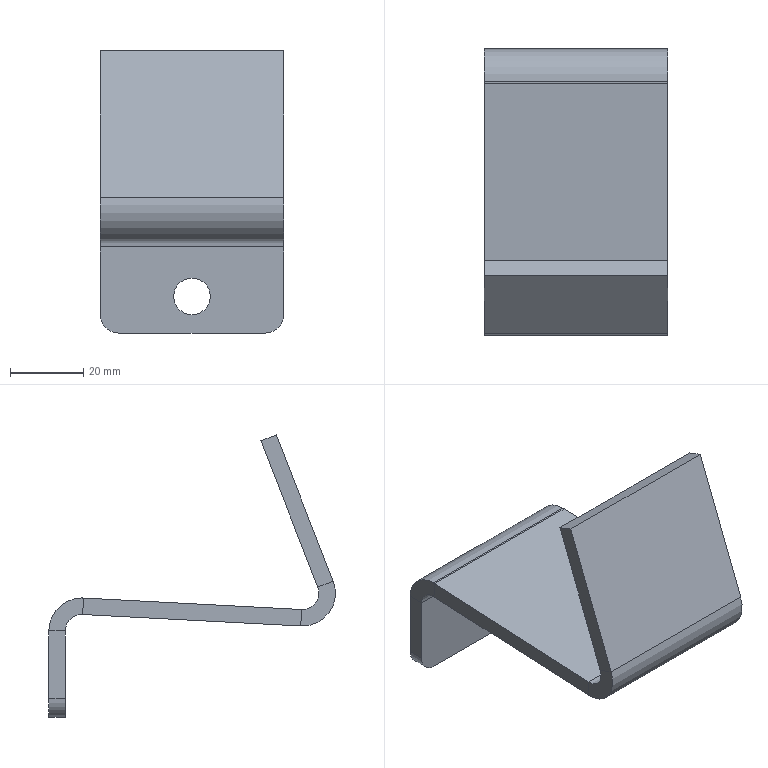Part | SolidWorks | features Fillet 1, FlatPattern 1, ICE 1, SMBaseFlange 1, SheetMetal 1 | 1 solid | 28 faces | box 50 x 78.274 x 77.035 mm | volume 33443 mm3 | plane 18 | cylinder 10 | commonest cylinder face diameters 10 x4 9 x3 18 x3
STEP:
#1=CARTESIAN_POINT('',(0.,-4.5,5.));
#2=VERTEX_POINT('',#1);
#3=CARTESIAN_POINT('',(0.,-4.5,15.));
#4=VERTEX_POINT('',#3);
#5=CARTESIAN_POINT('',(0.,-4.5,10.));
#6=DIRECTION('',(0.,1.,0.));
#7=DIRECTION('',(0.,0.,-1.));
#8=AXIS2_PLACEMENT_3D('',#5,#6,#7);
#9=CIRCLE('',#8,5.);
#10=EDGE_CURVE('',#2,#4,#9,.T.);
#11=ORIENTED_EDGE('',*,*,#10,.F.);
#12=CARTESIAN_POINT('',(0.,0.,5.));
#13=VERTEX_POINT('',#12);
#14=CARTESIAN_POINT('',(0.,-78.275,5.));
#15=DIRECTION('',(0.,1.,0.));
#16=VECTOR('',#15,1000.);
#17=LINE('',#14,#16);
#18=EDGE_CURVE('',#2,#13,#17,.T.);
#19=ORIENTED_EDGE('',*,*,#18,.T.);
#20=CARTESIAN_POINT('',(0.,0.,15.));
#21=VERTEX_POINT('',#20);
#22=CARTESIAN_POINT('',(0.,0.,10.));
#23=DIRECTION('',(0.,1.,0.));
#24=DIRECTION('',(0.,0.,1.));
#25=AXIS2_PLACEMENT_3D('',#22,#23,#24);
#26=CIRCLE('',#25,5.);
#27=EDGE_CURVE('',#13,#21,#26,.T.);
#28=ORIENTED_EDGE('',*,*,#27,.T.);
#29=CARTESIAN_POINT('',(0.,-78.275,15.));
#30=DIRECTION('',(0.,1.,0.));
#31=VECTOR('',#30,1000.);
#32=LINE('',#29,#31);
#33=EDGE_CURVE('',#4,#21,#32,.T.);
#34=ORIENTED_EDGE('',*,*,#33,.F.);
#35=EDGE_LOOP('',(#11,#19,#28,#34));
#36=FACE_OUTER_BOUND('',#35,.T.);
#37=CARTESIAN_POINT('',(0.,-78.275,10.));
#38=DIRECTION('',(0.,1.,0.));
#39=DIRECTION('',(0.,0.,1.));
#40=AXIS2_PLACEMENT_3D('',#37,#38,#39);
#41=CYLINDRICAL_SURFACE('',#40,5.);
#42=ADVANCED_FACE('',(#36),#41,.F.);
#43=CARTESIAN_POINT('',(25.,-9.,32.514));
#44=VERTEX_POINT('',#43);
#45=CARTESIAN_POINT('',(25.,-9.473,32.501));
#46=VERTEX_POINT('',#45);
#47=CARTESIAN_POINT('',(25.,-9.,23.514));
#48=DIRECTION('',(1.,0.,0.));
#49=DIRECTION('',(0.,0.,1.));
#50=AXIS2_PLACEMENT_3D('',#47,#48,#49);
#51=CIRCLE('',#50,9.);
#52=EDGE_CURVE('',#44,#46,#51,.T.);
#53=ORIENTED_EDGE('',*,*,#52,.F.);
#54=CARTESIAN_POINT('',(-25.,-9.,32.514));
#55=VERTEX_POINT('',#54);
#56=CARTESIAN_POINT('',(25.,-9.,32.514));
#57=DIRECTION('',(-1.,0.,0.));
#58=VECTOR('',#57,1000.);
#59=LINE('',#56,#58);
#60=EDGE_CURVE('',#44,#55,#59,.T.);
#61=ORIENTED_EDGE('',*,*,#60,.T.);
#62=CARTESIAN_POINT('',(-25.,-9.473,32.501));
#63=VERTEX_POINT('',#62);
#64=CARTESIAN_POINT('',(-25.,-9.,23.514));
#65=DIRECTION('',(1.,0.,0.));
#66=DIRECTION('',(0.,0.,1.));
#67=AXIS2_PLACEMENT_3D('',#64,#65,#66);
#68=CIRCLE('',#67,9.);
#69=EDGE_CURVE('',#55,#63,#68,.T.);
#70=ORIENTED_EDGE('',*,*,#69,.T.);
#71=CARTESIAN_POINT('',(25.,-9.473,32.501));
#72=DIRECTION('',(-1.,0.,0.));
#73=VECTOR('',#72,1000.);
#74=LINE('',#71,#73);
#75=EDGE_CURVE('',#46,#63,#74,.T.);
#76=ORIENTED_EDGE('',*,*,#75,.F.);
#77=EDGE_LOOP('',(#53,#61,#70,#76));
#78=FACE_OUTER_BOUND('',#77,.T.);
#79=CARTESIAN_POINT('',(25.,-9.,23.514));
#80=DIRECTION('',(-1.,0.,0.));
#81=DIRECTION('',(0.,0.,1.));
#82=AXIS2_PLACEMENT_3D('',#79,#80,#81);
#83=CYLINDRICAL_SURFACE('',#82,9.);
#84=ADVANCED_FACE('',(#78),#83,.T.);
#85=CARTESIAN_POINT('',(25.,-4.5,23.514));
#86=VERTEX_POINT('',#85);
#87=CARTESIAN_POINT('',(25.,-9.,28.014));
#88=VERTEX_POINT('',#87);
#89=CARTESIAN_POINT('',(25.,-9.,23.514));
#90=DIRECTION('',(1.,0.,0.));
#91=DIRECTION('',(0.,0.,-1.));
#92=AXIS2_PLACEMENT_3D('',#89,#90,#91);
#93=CIRCLE('',#92,4.5);
#94=EDGE_CURVE('',#86,#88,#93,.T.);
#95=ORIENTED_EDGE('',*,*,#94,.T.);
#96=CARTESIAN_POINT('',(-25.,-9.,28.014));
#97=VERTEX_POINT('',#96);
#98=CARTESIAN_POINT('',(25.,-9.,28.014));
#99=DIRECTION('',(-1.,0.,0.));
#100=VECTOR('',#99,1000.);
#101=LINE('',#98,#100);
#102=EDGE_CURVE('',#88,#97,#101,.T.);
#103=ORIENTED_EDGE('',*,*,#102,.T.);
#104=CARTESIAN_POINT('',(-25.,-4.5,23.514));
#105=VERTEX_POINT('',#104);
#106=CARTESIAN_POINT('',(-25.,-9.,23.514));
#107=DIRECTION('',(1.,0.,0.));
#108=DIRECTION('',(0.,0.,-1.));
#109=AXIS2_PLACEMENT_3D('',#106,#107,#108);
#110=CIRCLE('',#109,4.5);
#111=EDGE_CURVE('',#105,#97,#110,.T.);
#112=ORIENTED_EDGE('',*,*,#111,.F.);
#113=CARTESIAN_POINT('',(25.,-4.5,23.514));
#114=DIRECTION('',(-1.,0.,0.));
#115=VECTOR('',#114,1000.);
#116=LINE('',#113,#115);
#117=EDGE_CURVE('',#86,#105,#116,.T.);
#118=ORIENTED_EDGE('',*,*,#117,.F.);
#119=EDGE_LOOP('',(#95,#103,#112,#118));
#120=FACE_OUTER_BOUND('',#119,.T.);
#121=CARTESIAN_POINT('',(25.,-9.,23.514));
#122=DIRECTION('',(-1.,0.,0.));
#123=DIRECTION('',(0.,0.,1.));
#124=AXIS2_PLACEMENT_3D('',#121,#122,#123);
#125=CYLINDRICAL_SURFACE('',#124,4.5);
#126=ADVANCED_FACE('',(#120),#125,.F.);
#127=CARTESIAN_POINT('',(25.,0.,23.514));
#128=VERTEX_POINT('',#127);
#129=CARTESIAN_POINT('',(25.,0.,23.514));
#130=DIRECTION('',(0.,-1.,0.));
#131=VECTOR('',#130,1000.);
#132=LINE('',#129,#131);
#133=EDGE_CURVE('',#128,#86,#132,.T.);
#134=ORIENTED_EDGE('',*,*,#133,.F.);
#135=CARTESIAN_POINT('',(25.,-9.,23.514));
#136=DIRECTION('',(1.,0.,0.));
#137=DIRECTION('',(0.,0.,1.));
#138=AXIS2_PLACEMENT_3D('',#135,#136,#137);
#139=CIRCLE('',#138,9.);
#140=EDGE_CURVE('',#128,#44,#139,.T.);
#141=ORIENTED_EDGE('',*,*,#140,.T.);
#142=ORIENTED_EDGE('',*,*,#52,.T.);
#143=CARTESIAN_POINT('',(25.,-9.237,28.008));
#144=VERTEX_POINT('',#143);
#145=CARTESIAN_POINT('',(25.,-9.237,28.008));
#146=DIRECTION('',(0.,-0.05256,0.9986));
#147=VECTOR('',#146,1000.);
#148=LINE('',#145,#147);
#149=EDGE_CURVE('',#144,#46,#148,.T.);
#150=ORIENTED_EDGE('',*,*,#149,.F.);
#151=CARTESIAN_POINT('',(25.,-9.,23.514));
#152=DIRECTION('',(1.,0.,0.));
#153=DIRECTION('',(0.,0.,-1.));
#154=AXIS2_PLACEMENT_3D('',#151,#152,#153);
#155=CIRCLE('',#154,4.5);
#156=EDGE_CURVE('',#88,#144,#155,.T.);
#157=ORIENTED_EDGE('',*,*,#156,.F.);
#158=ORIENTED_EDGE('',*,*,#94,.F.);
#159=EDGE_LOOP('',(#134,#141,#142,#150,#157,#158));
#160=FACE_OUTER_BOUND('',#159,.T.);
#161=CARTESIAN_POINT('',(25.,0.,23.514));
#162=DIRECTION('',(1.,0.,0.));
#163=DIRECTION('',(0.,0.,-1.));
#164=AXIS2_PLACEMENT_3D('',#161,#162,#163);
#165=PLANE('',#164);
#166=ADVANCED_FACE('',(#160),#165,.T.);
#167=CARTESIAN_POINT('',(25.,-4.5,5.));
#168=VERTEX_POINT('',#167);
#169=CARTESIAN_POINT('',(25.,-4.5,0.));
#170=DIRECTION('',(0.,0.,1.));
#171=VECTOR('',#170,1000.);
#172=LINE('',#169,#171);
#173=EDGE_CURVE('',#168,#86,#172,.T.);
#174=ORIENTED_EDGE('',*,*,#173,.F.);
#175=CARTESIAN_POINT('',(25.,0.,5.));
#176=VERTEX_POINT('',#175);
#177=CARTESIAN_POINT('',(25.,-9.237,5.));
#178=DIRECTION('',(0.,1.,0.));
#179=VECTOR('',#178,1000.);
#180=LINE('',#177,#179);
#181=EDGE_CURVE('',#168,#176,#180,.T.);
#182=ORIENTED_EDGE('',*,*,#181,.T.);
#183=CARTESIAN_POINT('',(25.,0.,0.));
#184=DIRECTION('',(0.,0.,1.));
#185=VECTOR('',#184,1000.);
#186=LINE('',#183,#185);
#187=EDGE_CURVE('',#176,#128,#186,.T.);
#188=ORIENTED_EDGE('',*,*,#187,.T.);
#189=ORIENTED_EDGE('',*,*,#133,.T.);
#190=EDGE_LOOP('',(#174,#182,#188,#189));
#191=FACE_OUTER_BOUND('',#190,.T.);
#192=CARTESIAN_POINT('',(25.,-9.237,28.008));
#193=DIRECTION('',(1.,0.,0.));
#194=DIRECTION('',(0.,0.,-1.));
#195=AXIS2_PLACEMENT_3D('',#192,#193,#194);
#196=PLANE('',#195);
#197=ADVANCED_FACE('',(#191),#196,.T.);
#198=CARTESIAN_POINT('',(-25.,-9.237,28.008));
#199=VERTEX_POINT('',#198);
#200=CARTESIAN_POINT('',(-25.,-9.473,32.501));
#201=DIRECTION('',(0.,0.05256,-0.9986));
#202=VECTOR('',#201,1000.);
#203=LINE('',#200,#202);
#204=EDGE_CURVE('',#63,#199,#203,.T.);
#205=ORIENTED_EDGE('',*,*,#204,.F.);
#206=ORIENTED_EDGE('',*,*,#69,.F.);
#207=CARTESIAN_POINT('',(-25.,0.,23.514));
#208=VERTEX_POINT('',#207);
#209=CARTESIAN_POINT('',(-25.,-9.,23.514));
#210=DIRECTION('',(1.,0.,0.));
#211=DIRECTION('',(0.,0.,1.));
#212=AXIS2_PLACEMENT_3D('',#209,#210,#211);
#213=CIRCLE('',#212,9.);
#214=EDGE_CURVE('',#208,#55,#213,.T.);
#215=ORIENTED_EDGE('',*,*,#214,.F.);
#216=CARTESIAN_POINT('',(-25.,-4.5,23.514));
#217=DIRECTION('',(0.,1.,0.));
#218=VECTOR('',#217,1000.);
#219=LINE('',#216,#218);
#220=EDGE_CURVE('',#105,#208,#219,.T.);
#221=ORIENTED_EDGE('',*,*,#220,.F.);
#222=ORIENTED_EDGE('',*,*,#111,.T.);
#223=CARTESIAN_POINT('',(-25.,-9.,23.514));
#224=DIRECTION('',(1.,0.,0.));
#225=DIRECTION('',(0.,0.,-1.));
#226=AXIS2_PLACEMENT_3D('',#223,#224,#225);
#227=CIRCLE('',#226,4.5);
#228=EDGE_CURVE('',#97,#199,#227,.T.);
#229=ORIENTED_EDGE('',*,*,#228,.T.);
#230=EDGE_LOOP('',(#205,#206,#215,#221,#222,#229));
#231=FACE_OUTER_BOUND('',#230,.T.);
#232=CARTESIAN_POINT('',(-25.,-9.473,32.501));
#233=DIRECTION('',(-1.,0.,0.));
#234=DIRECTION('',(0.,0.,1.));
#235=AXIS2_PLACEMENT_3D('',#232,#233,#234);
#236=PLANE('',#235);
#237=ADVANCED_FACE('',(#231),#236,.T.);
#238=CARTESIAN_POINT('',(-25.,-69.037,29.366));
#239=VERTEX_POINT('',#238);
#240=CARTESIAN_POINT('',(-25.,0.,33.));
#241=DIRECTION('',(0.,-0.9986,-0.05256));
#242=VECTOR('',#241,1000.);
#243=LINE('',#240,#242);
#244=EDGE_CURVE('',#63,#239,#243,.T.);
#245=ORIENTED_EDGE('',*,*,#244,.F.);
#246=ORIENTED_EDGE('',*,*,#204,.T.);
#247=CARTESIAN_POINT('',(-25.,-68.801,24.873));
#248=VERTEX_POINT('',#247);
#249=CARTESIAN_POINT('',(-25.,0.2365,28.506));
#250=DIRECTION('',(0.,-0.9986,-0.05256));
#251=VECTOR('',#250,1000.);
#252=LINE('',#249,#251);
#253=EDGE_CURVE('',#199,#248,#252,.T.);
#254=ORIENTED_EDGE('',*,*,#253,.T.);
#255=CARTESIAN_POINT('',(-25.,-68.801,24.873));
#256=DIRECTION('',(0.,-0.05256,0.9986));
#257=VECTOR('',#256,1000.);
#258=LINE('',#255,#257);
#259=EDGE_CURVE('',#248,#239,#258,.T.);
#260=ORIENTED_EDGE('',*,*,#259,.T.);
#261=EDGE_LOOP('',(#245,#246,#254,#260));
#262=FACE_OUTER_BOUND('',#261,.T.);
#263=CARTESIAN_POINT('',(-25.,-4.5,23.514));
#264=DIRECTION('',(-1.,0.,0.));
#265=DIRECTION('',(0.,0.,1.));
#266=AXIS2_PLACEMENT_3D('',#263,#264,#265);
#267=PLANE('',#266);
#268=ADVANCED_FACE('',(#262),#267,.T.);
#269=CARTESIAN_POINT('',(25.,-69.037,29.366));
#270=VERTEX_POINT('',#269);
#271=CARTESIAN_POINT('',(25.,-68.801,24.873));
#272=VERTEX_POINT('',#271);
#273=CARTESIAN_POINT('',(25.,-69.037,29.366));
#274=DIRECTION('',(0.,0.05256,-0.9986));
#275=VECTOR('',#274,1000.);
#276=LINE('',#273,#275);
#277=EDGE_CURVE('',#270,#272,#276,.T.);
#278=ORIENTED_EDGE('',*,*,#277,.F.);
#279=CARTESIAN_POINT('',(25.,-73.466,35.496));
#280=VERTEX_POINT('',#279);
#281=CARTESIAN_POINT('',(25.,-69.274,33.86));
#282=DIRECTION('',(-1.,0.,0.));
#283=DIRECTION('',(0.,0.,-1.));
#284=AXIS2_PLACEMENT_3D('',#281,#282,#283);
#285=CIRCLE('',#284,4.5);
#286=EDGE_CURVE('',#270,#280,#285,.T.);
#287=ORIENTED_EDGE('',*,*,#286,.T.);
#288=CARTESIAN_POINT('',(25.,-77.658,37.131));
#289=VERTEX_POINT('',#288);
#290=CARTESIAN_POINT('',(25.,-77.658,37.131));
#291=DIRECTION('',(0.,0.9316,-0.3634));
#292=VECTOR('',#291,1000.);
#293=LINE('',#290,#292);
#294=EDGE_CURVE('',#289,#280,#293,.T.);
#295=ORIENTED_EDGE('',*,*,#294,.F.);
#296=CARTESIAN_POINT('',(25.,-69.274,33.86));
#297=DIRECTION('',(-1.,0.,0.));
#298=DIRECTION('',(0.,0.,-1.));
#299=AXIS2_PLACEMENT_3D('',#296,#297,#298);
#300=CIRCLE('',#299,9.);
#301=EDGE_CURVE('',#272,#289,#300,.T.);
#302=ORIENTED_EDGE('',*,*,#301,.F.);
#303=EDGE_LOOP('',(#278,#287,#295,#302));
#304=FACE_OUTER_BOUND('',#303,.T.);
#305=CARTESIAN_POINT('',(25.,-69.037,29.366));
#306=DIRECTION('',(1.,0.,0.));
#307=DIRECTION('',(0.,0.,-1.));
#308=AXIS2_PLACEMENT_3D('',#305,#306,#307);
#309=PLANE('',#308);
#310=ADVANCED_FACE('',(#304),#309,.T.);
#311=CARTESIAN_POINT('',(25.,0.,33.));
#312=DIRECTION('',(0.,-0.9986,-0.05256));
#313=VECTOR('',#312,1000.);
#314=LINE('',#311,#313);
#315=EDGE_CURVE('',#46,#270,#314,.T.);
#316=ORIENTED_EDGE('',*,*,#315,.T.);
#317=ORIENTED_EDGE('',*,*,#277,.T.);
#318=CARTESIAN_POINT('',(25.,0.2365,28.506));
#319=DIRECTION('',(0.,-0.9986,-0.05256));
#320=VECTOR('',#319,1000.);
#321=LINE('',#318,#320);
#322=EDGE_CURVE('',#144,#272,#321,.T.);
#323=ORIENTED_EDGE('',*,*,#322,.F.);
#324=ORIENTED_EDGE('',*,*,#149,.T.);
#325=EDGE_LOOP('',(#316,#317,#323,#324));
#326=FACE_OUTER_BOUND('',#325,.T.);
#327=CARTESIAN_POINT('',(25.,-77.658,37.131));
#328=DIRECTION('',(1.,0.,0.));
#329=DIRECTION('',(0.,0.,-1.));
#330=AXIS2_PLACEMENT_3D('',#327,#328,#329);
#331=PLANE('',#330);
#332=ADVANCED_FACE('',(#326),#331,.T.);
#333=CARTESIAN_POINT('',(-25.,-73.466,35.496));
#334=VERTEX_POINT('',#333);
#335=CARTESIAN_POINT('',(-25.,-77.658,37.131));
#336=VERTEX_POINT('',#335);
#337=CARTESIAN_POINT('',(-25.,-73.466,35.496));
#338=DIRECTION('',(0.,-0.9316,0.3634));
#339=VECTOR('',#338,1000.);
#340=LINE('',#337,#339);
#341=EDGE_CURVE('',#334,#336,#340,.T.);
#342=ORIENTED_EDGE('',*,*,#341,.F.);
#343=CARTESIAN_POINT('',(-25.,-69.274,33.86));
#344=DIRECTION('',(-1.,0.,0.));
#345=DIRECTION('',(0.,0.,-1.));
#346=AXIS2_PLACEMENT_3D('',#343,#344,#345);
#347=CIRCLE('',#346,4.5);
#348=EDGE_CURVE('',#239,#334,#347,.T.);
#349=ORIENTED_EDGE('',*,*,#348,.F.);
#350=ORIENTED_EDGE('',*,*,#259,.F.);
#351=CARTESIAN_POINT('',(-25.,-69.274,33.86));
#352=DIRECTION('',(-1.,0.,0.));
#353=DIRECTION('',(0.,0.,-1.));
#354=AXIS2_PLACEMENT_3D('',#351,#352,#353);
#355=CIRCLE('',#354,9.);
#356=EDGE_CURVE('',#248,#336,#355,.T.);
#357=ORIENTED_EDGE('',*,*,#356,.T.);
#358=EDGE_LOOP('',(#342,#349,#350,#357));
#359=FACE_OUTER_BOUND('',#358,.T.);
#360=CARTESIAN_POINT('',(-25.,-73.466,35.496));
#361=DIRECTION('',(-1.,0.,0.));
#362=DIRECTION('',(0.,0.,1.));
#363=AXIS2_PLACEMENT_3D('',#360,#361,#362);
#364=PLANE('',#363);
#365=ADVANCED_FACE('',(#359),#364,.T.);
#366=CARTESIAN_POINT('',(-25.,-57.9,75.4));
#367=VERTEX_POINT('',#366);
#368=CARTESIAN_POINT('',(-25.,-76.,29.));
#369=DIRECTION('',(0.,0.3634,0.9316));
#370=VECTOR('',#369,1000.);
#371=LINE('',#368,#370);
#372=EDGE_CURVE('',#334,#367,#371,.T.);
#373=ORIENTED_EDGE('',*,*,#372,.F.);
#374=ORIENTED_EDGE('',*,*,#341,.T.);
#375=CARTESIAN_POINT('',(-25.,-62.092,77.035));
#376=VERTEX_POINT('',#375);
#377=CARTESIAN_POINT('',(-25.,-80.192,30.635));
#378=DIRECTION('',(0.,0.3634,0.9316));
#379=VECTOR('',#378,1000.);
#380=LINE('',#377,#379);
#381=EDGE_CURVE('',#336,#376,#380,.T.);
#382=ORIENTED_EDGE('',*,*,#381,.T.);
#383=CARTESIAN_POINT('',(-25.,-62.092,77.035));
#384=DIRECTION('',(0.,0.9316,-0.3634));
#385=VECTOR('',#384,1000.);
#386=LINE('',#383,#385);
#387=EDGE_CURVE('',#376,#367,#386,.T.);
#388=ORIENTED_EDGE('',*,*,#387,.T.);
#389=EDGE_LOOP('',(#373,#374,#382,#388));
#390=FACE_OUTER_BOUND('',#389,.T.);
#391=CARTESIAN_POINT('',(-25.,-68.801,24.873));
#392=DIRECTION('',(-1.,0.,0.));
#393=DIRECTION('',(0.,0.,1.));
#394=AXIS2_PLACEMENT_3D('',#391,#392,#393);
#395=PLANE('',#394);
#396=ADVANCED_FACE('',(#390),#395,.T.);
#397=ORIENTED_EDGE('',*,*,#372,.T.);
#398=CARTESIAN_POINT('',(25.,-57.9,75.4));
#399=VERTEX_POINT('',#398);
#400=CARTESIAN_POINT('',(25.,-57.9,75.4));
#401=DIRECTION('',(-1.,0.,0.));
#402=VECTOR('',#401,1000.);
#403=LINE('',#400,#402);
#404=EDGE_CURVE('',#399,#367,#403,.T.);
#405=ORIENTED_EDGE('',*,*,#404,.F.);
#406=CARTESIAN_POINT('',(25.,-76.,29.));
#407=DIRECTION('',(0.,0.3634,0.9316));
#408=VECTOR('',#407,1000.);
#409=LINE('',#406,#408);
#410=EDGE_CURVE('',#280,#399,#409,.T.);
#411=ORIENTED_EDGE('',*,*,#410,.F.);
#412=CARTESIAN_POINT('',(25.,-73.466,35.496));
#413=DIRECTION('',(-1.,0.,0.));
#414=VECTOR('',#413,1000.);
#415=LINE('',#412,#414);
#416=EDGE_CURVE('',#280,#334,#415,.T.);
#417=ORIENTED_EDGE('',*,*,#416,.T.);
#418=EDGE_LOOP('',(#397,#405,#411,#417));
#419=FACE_OUTER_BOUND('',#418,.T.);
#420=CARTESIAN_POINT('',(25.,-76.,29.));
#421=DIRECTION('',(0.,-0.9316,0.3634));
#422=DIRECTION('',(0.,-0.3634,-0.9316));
#423=AXIS2_PLACEMENT_3D('',#420,#421,#422);
#424=PLANE('',#423);
#425=ADVANCED_FACE('',(#419),#424,.F.);
#426=ORIENTED_EDGE('',*,*,#387,.F.);
#427=CARTESIAN_POINT('',(25.,-62.092,77.035));
#428=VERTEX_POINT('',#427);
#429=CARTESIAN_POINT('',(25.,-62.092,77.035));
#430=DIRECTION('',(-1.,0.,0.));
#431=VECTOR('',#430,1000.);
#432=LINE('',#429,#431);
#433=EDGE_CURVE('',#428,#376,#432,.T.);
#434=ORIENTED_EDGE('',*,*,#433,.F.);
#435=CARTESIAN_POINT('',(25.,-62.092,77.035));
#436=DIRECTION('',(0.,0.9316,-0.3634));
#437=VECTOR('',#436,1000.);
#438=LINE('',#435,#437);
#439=EDGE_CURVE('',#428,#399,#438,.T.);
#440=ORIENTED_EDGE('',*,*,#439,.T.);
#441=ORIENTED_EDGE('',*,*,#404,.T.);
#442=EDGE_LOOP('',(#426,#434,#440,#441));
#443=FACE_OUTER_BOUND('',#442,.T.);
#444=CARTESIAN_POINT('',(25.,-62.092,77.035));
#445=DIRECTION('',(0.,0.3634,0.9316));
#446=DIRECTION('',(0.,-0.9316,0.3634));
#447=AXIS2_PLACEMENT_3D('',#444,#445,#446);
#448=PLANE('',#447);
#449=ADVANCED_FACE('',(#443),#448,.T.);
#450=ORIENTED_EDGE('',*,*,#381,.F.);
#451=CARTESIAN_POINT('',(25.,-77.658,37.131));
#452=DIRECTION('',(-1.,0.,0.));
#453=VECTOR('',#452,1000.);
#454=LINE('',#451,#453);
#455=EDGE_CURVE('',#289,#336,#454,.T.);
#456=ORIENTED_EDGE('',*,*,#455,.F.);
#457=CARTESIAN_POINT('',(25.,-80.192,30.635));
#458=DIRECTION('',(0.,0.3634,0.9316));
#459=VECTOR('',#458,1000.);
#460=LINE('',#457,#459);
#461=EDGE_CURVE('',#289,#428,#460,.T.);
#462=ORIENTED_EDGE('',*,*,#461,.T.);
#463=ORIENTED_EDGE('',*,*,#433,.T.);
#464=EDGE_LOOP('',(#450,#456,#462,#463));
#465=FACE_OUTER_BOUND('',#464,.T.);
#466=CARTESIAN_POINT('',(25.,-80.192,30.635));
#467=DIRECTION('',(0.,-0.9316,0.3634));
#468=DIRECTION('',(0.,-0.3634,-0.9316));
#469=AXIS2_PLACEMENT_3D('',#466,#467,#468);
#470=PLANE('',#469);
#471=ADVANCED_FACE('',(#465),#470,.T.);
#472=ORIENTED_EDGE('',*,*,#356,.F.);
#473=CARTESIAN_POINT('',(25.,-68.801,24.873));
#474=DIRECTION('',(-1.,0.,0.));
#475=VECTOR('',#474,1000.);
#476=LINE('',#473,#475);
#477=EDGE_CURVE('',#272,#248,#476,.T.);
#478=ORIENTED_EDGE('',*,*,#477,.F.);
#479=ORIENTED_EDGE('',*,*,#301,.T.);
#480=ORIENTED_EDGE('',*,*,#455,.T.);
#481=EDGE_LOOP('',(#472,#478,#479,#480));
#482=FACE_OUTER_BOUND('',#481,.T.);
#483=CARTESIAN_POINT('',(25.,-69.274,33.86));
#484=DIRECTION('',(-1.,0.,0.));
#485=DIRECTION('',(0.,0.,1.));
#486=AXIS2_PLACEMENT_3D('',#483,#484,#485);
#487=CYLINDRICAL_SURFACE('',#486,9.);
#488=ADVANCED_FACE('',(#482),#487,.T.);
#489=ORIENTED_EDGE('',*,*,#253,.F.);
#490=CARTESIAN_POINT('',(25.,-9.237,28.008));
#491=DIRECTION('',(-1.,0.,0.));
#492=VECTOR('',#491,1000.);
#493=LINE('',#490,#492);
#494=EDGE_CURVE('',#144,#199,#493,.T.);
#495=ORIENTED_EDGE('',*,*,#494,.F.);
#496=ORIENTED_EDGE('',*,*,#322,.T.);
#497=ORIENTED_EDGE('',*,*,#477,.T.);
#498=EDGE_LOOP('',(#489,#495,#496,#497));
#499=FACE_OUTER_BOUND('',#498,.T.);
#500=CARTESIAN_POINT('',(25.,0.2365,28.506));
#501=DIRECTION('',(0.,0.05256,-0.9986));
#502=DIRECTION('',(0.,0.9986,0.05256));
#503=AXIS2_PLACEMENT_3D('',#500,#501,#502);
#504=PLANE('',#503);
#505=ADVANCED_FACE('',(#499),#504,.T.);
#506=ORIENTED_EDGE('',*,*,#102,.F.);
#507=ORIENTED_EDGE('',*,*,#156,.T.);
#508=ORIENTED_EDGE('',*,*,#494,.T.);
#509=ORIENTED_EDGE('',*,*,#228,.F.);
#510=EDGE_LOOP('',(#506,#507,#508,#509));
#511=FACE_OUTER_BOUND('',#510,.T.);
#512=CARTESIAN_POINT('',(25.,-9.,23.514));
#513=DIRECTION('',(-1.,0.,0.));
#514=DIRECTION('',(0.,0.,1.));
#515=AXIS2_PLACEMENT_3D('',#512,#513,#514);
#516=CYLINDRICAL_SURFACE('',#515,4.5);
#517=ADVANCED_FACE('',(#511),#516,.F.);
#518=CARTESIAN_POINT('',(0.,-4.5,10.));
#519=DIRECTION('',(0.,1.,0.));
#520=DIRECTION('',(0.,0.,-1.));
#521=AXIS2_PLACEMENT_3D('',#518,#519,#520);
#522=CIRCLE('',#521,5.);
#523=EDGE_CURVE('',#4,#2,#522,.T.);
#524=ORIENTED_EDGE('',*,*,#523,.T.);
#525=ORIENTED_EDGE('',*,*,#10,.T.);
#526=EDGE_LOOP('',(#524,#525));
#527=FACE_BOUND('',#526,.T.);
#528=CARTESIAN_POINT('',(20.,-4.5,0.));
#529=VERTEX_POINT('',#528);
#530=CARTESIAN_POINT('',(-20.,-4.5,0.));
#531=VERTEX_POINT('',#530);
#532=CARTESIAN_POINT('',(25.,-4.5,0.));
#533=DIRECTION('',(-1.,0.,0.));
#534=VECTOR('',#533,1000.);
#535=LINE('',#532,#534);
#536=EDGE_CURVE('',#529,#531,#535,.T.);
#537=ORIENTED_EDGE('',*,*,#536,.F.);
#538=CARTESIAN_POINT('',(20.,-4.5,5.));
#539=DIRECTION('',(0.,-1.,0.));
#540=DIRECTION('',(0.,0.,-1.));
#541=AXIS2_PLACEMENT_3D('',#538,#539,#540);
#542=CIRCLE('',#541,5.);
#543=EDGE_CURVE('',#529,#168,#542,.T.);
#544=ORIENTED_EDGE('',*,*,#543,.T.);
#545=ORIENTED_EDGE('',*,*,#173,.T.);
#546=ORIENTED_EDGE('',*,*,#117,.T.);
#547=CARTESIAN_POINT('',(-25.,-4.5,5.));
#548=VERTEX_POINT('',#547);
#549=CARTESIAN_POINT('',(-25.,-4.5,0.));
#550=DIRECTION('',(0.,0.,1.));
#551=VECTOR('',#550,1000.);
#552=LINE('',#549,#551);
#553=EDGE_CURVE('',#548,#105,#552,.T.);
#554=ORIENTED_EDGE('',*,*,#553,.F.);
#555=CARTESIAN_POINT('',(-20.,-4.5,5.));
#556=DIRECTION('',(0.,-1.,0.));
#557=DIRECTION('',(0.,0.,-1.));
#558=AXIS2_PLACEMENT_3D('',#555,#556,#557);
#559=CIRCLE('',#558,5.);
#560=EDGE_CURVE('',#548,#531,#559,.T.);
#561=ORIENTED_EDGE('',*,*,#560,.T.);
#562=EDGE_LOOP('',(#537,#544,#545,#546,#554,#561));
#563=FACE_OUTER_BOUND('',#562,.T.);
#564=CARTESIAN_POINT('',(25.,-4.5,0.));
#565=DIRECTION('',(0.,-1.,0.));
#566=DIRECTION('',(0.,0.,-1.));
#567=AXIS2_PLACEMENT_3D('',#564,#565,#566);
#568=PLANE('',#567);
#569=ADVANCED_FACE('',(#527,#563),#568,.T.);
#570=CARTESIAN_POINT('',(20.,0.,0.));
#571=VERTEX_POINT('',#570);
#572=CARTESIAN_POINT('',(-20.,0.,0.));
#573=VERTEX_POINT('',#572);
#574=CARTESIAN_POINT('',(25.,0.,0.));
#575=DIRECTION('',(-1.,0.,0.));
#576=VECTOR('',#575,1000.);
#577=LINE('',#574,#576);
#578=EDGE_CURVE('',#571,#573,#577,.T.);
#579=ORIENTED_EDGE('',*,*,#578,.F.);
#580=CARTESIAN_POINT('',(20.,0.,0.));
#581=DIRECTION('',(0.,-1.,0.));
#582=VECTOR('',#581,1000.);
#583=LINE('',#580,#582);
#584=EDGE_CURVE('',#571,#529,#583,.T.);
#585=ORIENTED_EDGE('',*,*,#584,.T.);
#586=ORIENTED_EDGE('',*,*,#536,.T.);
#587=CARTESIAN_POINT('',(-20.,0.,0.));
#588=DIRECTION('',(0.,1.,0.));
#589=VECTOR('',#588,1000.);
#590=LINE('',#587,#589);
#591=EDGE_CURVE('',#531,#573,#590,.T.);
#592=ORIENTED_EDGE('',*,*,#591,.T.);
#593=EDGE_LOOP('',(#579,#585,#586,#592));
#594=FACE_OUTER_BOUND('',#593,.T.);
#595=CARTESIAN_POINT('',(25.,0.,0.));
#596=DIRECTION('',(0.,0.,-1.));
#597=DIRECTION('',(-1.,0.,0.));
#598=AXIS2_PLACEMENT_3D('',#595,#596,#597);
#599=PLANE('',#598);
#600=ADVANCED_FACE('',(#594),#599,.T.);
#601=CARTESIAN_POINT('',(0.,0.,10.));
#602=DIRECTION('',(0.,1.,0.));
#603=DIRECTION('',(0.,0.,1.));
#604=AXIS2_PLACEMENT_3D('',#601,#602,#603);
#605=CIRCLE('',#604,5.);
#606=EDGE_CURVE('',#21,#13,#605,.T.);
#607=ORIENTED_EDGE('',*,*,#606,.F.);
#608=ORIENTED_EDGE('',*,*,#27,.F.);
#609=EDGE_LOOP('',(#607,#608));
#610=FACE_BOUND('',#609,.T.);
#611=ORIENTED_EDGE('',*,*,#187,.F.);
#612=CARTESIAN_POINT('',(20.,0.,5.));
#613=DIRECTION('',(0.,1.,0.));
#614=DIRECTION('',(0.,0.,-1.));
#615=AXIS2_PLACEMENT_3D('',#612,#613,#614);
#616=CIRCLE('',#615,5.);
#617=EDGE_CURVE('',#176,#571,#616,.T.);
#618=ORIENTED_EDGE('',*,*,#617,.T.);
#619=ORIENTED_EDGE('',*,*,#578,.T.);
#620=CARTESIAN_POINT('',(-25.,0.,5.));
#621=VERTEX_POINT('',#620);
#622=CARTESIAN_POINT('',(-20.,0.,5.));
#623=DIRECTION('',(0.,1.,0.));
#624=DIRECTION('',(0.,0.,-1.));
#625=AXIS2_PLACEMENT_3D('',#622,#623,#624);
#626=CIRCLE('',#625,5.);
#627=EDGE_CURVE('',#573,#621,#626,.T.);
#628=ORIENTED_EDGE('',*,*,#627,.T.);
#629=CARTESIAN_POINT('',(-25.,0.,0.));
#630=DIRECTION('',(0.,0.,1.));
#631=VECTOR('',#630,1000.);
#632=LINE('',#629,#631);
#633=EDGE_CURVE('',#621,#208,#632,.T.);
#634=ORIENTED_EDGE('',*,*,#633,.T.);
#635=CARTESIAN_POINT('',(25.,0.,23.514));
#636=DIRECTION('',(-1.,0.,0.));
#637=VECTOR('',#636,1000.);
#638=LINE('',#635,#637);
#639=EDGE_CURVE('',#128,#208,#638,.T.);
#640=ORIENTED_EDGE('',*,*,#639,.F.);
#641=EDGE_LOOP('',(#611,#618,#619,#628,#634,#640));
#642=FACE_OUTER_BOUND('',#641,.T.);
#643=CARTESIAN_POINT('',(25.,0.,0.));
#644=DIRECTION('',(0.,-1.,0.));
#645=DIRECTION('',(0.,0.,-1.));
#646=AXIS2_PLACEMENT_3D('',#643,#644,#645);
#647=PLANE('',#646);
#648=ADVANCED_FACE('',(#610,#642),#647,.F.);
#649=ORIENTED_EDGE('',*,*,#60,.F.);
#650=ORIENTED_EDGE('',*,*,#140,.F.);
#651=ORIENTED_EDGE('',*,*,#639,.T.);
#652=ORIENTED_EDGE('',*,*,#214,.T.);
#653=EDGE_LOOP('',(#649,#650,#651,#652));
#654=FACE_OUTER_BOUND('',#653,.T.);
#655=CARTESIAN_POINT('',(25.,-9.,23.514));
#656=DIRECTION('',(-1.,0.,0.));
#657=DIRECTION('',(0.,0.,1.));
#658=AXIS2_PLACEMENT_3D('',#655,#656,#657);
#659=CYLINDRICAL_SURFACE('',#658,9.);
#660=ADVANCED_FACE('',(#654),#659,.T.);
#661=ORIENTED_EDGE('',*,*,#244,.T.);
#662=CARTESIAN_POINT('',(25.,-69.037,29.366));
#663=DIRECTION('',(-1.,0.,0.));
#664=VECTOR('',#663,1000.);
#665=LINE('',#662,#664);
#666=EDGE_CURVE('',#270,#239,#665,.T.);
#667=ORIENTED_EDGE('',*,*,#666,.F.);
#668=ORIENTED_EDGE('',*,*,#315,.F.);
#669=ORIENTED_EDGE('',*,*,#75,.T.);
#670=EDGE_LOOP('',(#661,#667,#668,#669));
#671=FACE_OUTER_BOUND('',#670,.T.);
#672=CARTESIAN_POINT('',(25.,0.,33.));
#673=DIRECTION('',(0.,0.05256,-0.9986));
#674=DIRECTION('',(0.,0.9986,0.05256));
#675=AXIS2_PLACEMENT_3D('',#672,#673,#674);
#676=PLANE('',#675);
#677=ADVANCED_FACE('',(#671),#676,.F.);
#678=ORIENTED_EDGE('',*,*,#348,.T.);
#679=ORIENTED_EDGE('',*,*,#416,.F.);
#680=ORIENTED_EDGE('',*,*,#286,.F.);
#681=ORIENTED_EDGE('',*,*,#666,.T.);
#682=EDGE_LOOP('',(#678,#679,#680,#681));
#683=FACE_OUTER_BOUND('',#682,.T.);
#684=CARTESIAN_POINT('',(25.,-69.274,33.86));
#685=DIRECTION('',(-1.,0.,0.));
#686=DIRECTION('',(0.,0.,1.));
#687=AXIS2_PLACEMENT_3D('',#684,#685,#686);
#688=CYLINDRICAL_SURFACE('',#687,4.5);
#689=ADVANCED_FACE('',(#683),#688,.F.);
#690=ORIENTED_EDGE('',*,*,#410,.T.);
#691=ORIENTED_EDGE('',*,*,#439,.F.);
#692=ORIENTED_EDGE('',*,*,#461,.F.);
#693=ORIENTED_EDGE('',*,*,#294,.T.);
#694=EDGE_LOOP('',(#690,#691,#692,#693));
#695=FACE_OUTER_BOUND('',#694,.T.);
#696=CARTESIAN_POINT('',(25.,-69.274,33.86));
#697=DIRECTION('',(1.,0.,0.));
#698=DIRECTION('',(0.,0.,-1.));
#699=AXIS2_PLACEMENT_3D('',#696,#697,#698);
#700=PLANE('',#699);
#701=ADVANCED_FACE('',(#695),#700,.T.);
#702=ORIENTED_EDGE('',*,*,#633,.F.);
#703=CARTESIAN_POINT('',(-25.,-4.5,5.));
#704=DIRECTION('',(0.,-1.,0.));
#705=VECTOR('',#704,1000.);
#706=LINE('',#703,#705);
#707=EDGE_CURVE('',#621,#548,#706,.T.);
#708=ORIENTED_EDGE('',*,*,#707,.T.);
#709=ORIENTED_EDGE('',*,*,#553,.T.);
#710=ORIENTED_EDGE('',*,*,#220,.T.);
#711=EDGE_LOOP('',(#702,#708,#709,#710));
#712=FACE_OUTER_BOUND('',#711,.T.);
#713=CARTESIAN_POINT('',(-25.,-69.274,33.86));
#714=DIRECTION('',(1.,0.,0.));
#715=DIRECTION('',(0.,0.,-1.));
#716=AXIS2_PLACEMENT_3D('',#713,#714,#715);
#717=PLANE('',#716);
#718=ADVANCED_FACE('',(#712),#717,.F.);
#719=ORIENTED_EDGE('',*,*,#18,.F.);
#720=ORIENTED_EDGE('',*,*,#523,.F.);
#721=ORIENTED_EDGE('',*,*,#33,.T.);
#722=ORIENTED_EDGE('',*,*,#606,.T.);
#723=EDGE_LOOP('',(#719,#720,#721,#722));
#724=FACE_OUTER_BOUND('',#723,.T.);
#725=CARTESIAN_POINT('',(0.,-78.275,10.));
#726=DIRECTION('',(0.,1.,0.));
#727=DIRECTION('',(0.,0.,1.));
#728=AXIS2_PLACEMENT_3D('',#725,#726,#727);
#729=CYLINDRICAL_SURFACE('',#728,5.);
#730=ADVANCED_FACE('',(#724),#729,.F.);
#731=ORIENTED_EDGE('',*,*,#617,.F.);
#732=ORIENTED_EDGE('',*,*,#181,.F.);
#733=ORIENTED_EDGE('',*,*,#543,.F.);
#734=ORIENTED_EDGE('',*,*,#584,.F.);
#735=EDGE_LOOP('',(#731,#732,#733,#734));
#736=FACE_OUTER_BOUND('',#735,.T.);
#737=CARTESIAN_POINT('',(20.,0.,5.));
#738=DIRECTION('',(0.,-1.,0.));
#739=DIRECTION('',(0.,0.,-1.));
#740=AXIS2_PLACEMENT_3D('',#737,#738,#739);
#741=CYLINDRICAL_SURFACE('',#740,5.);
#742=ADVANCED_FACE('',(#736),#741,.T.);
#743=ORIENTED_EDGE('',*,*,#627,.F.);
#744=ORIENTED_EDGE('',*,*,#591,.F.);
#745=ORIENTED_EDGE('',*,*,#560,.F.);
#746=ORIENTED_EDGE('',*,*,#707,.F.);
#747=EDGE_LOOP('',(#743,#744,#745,#746));
#748=FACE_OUTER_BOUND('',#747,.T.);
#749=CARTESIAN_POINT('',(-20.,-69.274,5.));
#750=DIRECTION('',(0.,1.,0.));
#751=DIRECTION('',(0.,0.,1.));
#752=AXIS2_PLACEMENT_3D('',#749,#750,#751);
#753=CYLINDRICAL_SURFACE('',#752,5.);
#754=ADVANCED_FACE('',(#748),#753,.T.);
#755=CLOSED_SHELL('',(#42,#84,#126,#166,#197,#237,#268,#310,#332,#365,#396,#425,#449,#471,#488,#505,#517,#569,#600,#648,#660,#677,#689,#701,#718,#730,#742,#754));
#756=MANIFOLD_SOLID_BREP('',#755);
#757=CARTESIAN_POINT('',(0.,0.,0.));
#758=DIRECTION('',(0.,0.,1.));
#759=DIRECTION('',(1.,0.,0.));
#760=AXIS2_PLACEMENT_3D('',#757,#758,#759);
#761=(LENGTH_UNIT()NAMED_UNIT(*)SI_UNIT(.MILLI.,.METRE.));
#762=UNCERTAINTY_MEASURE_WITH_UNIT(LENGTH_MEASURE(0.00001),#761,'','');
#763=(NAMED_UNIT(*)PLANE_ANGLE_UNIT()SI_UNIT($,.RADIAN.));
#764=(NAMED_UNIT(*)SI_UNIT($,.STERADIAN.)SOLID_ANGLE_UNIT());
#765=(GEOMETRIC_REPRESENTATION_CONTEXT(3)GLOBAL_UNCERTAINTY_ASSIGNED_CONTEXT((#762))GLOBAL_UNIT_ASSIGNED_CONTEXT((#761,#763,#764))REPRESENTATION_CONTEXT('',''));
#766=ADVANCED_BREP_SHAPE_REPRESENTATION('',(#756,#760),#765);